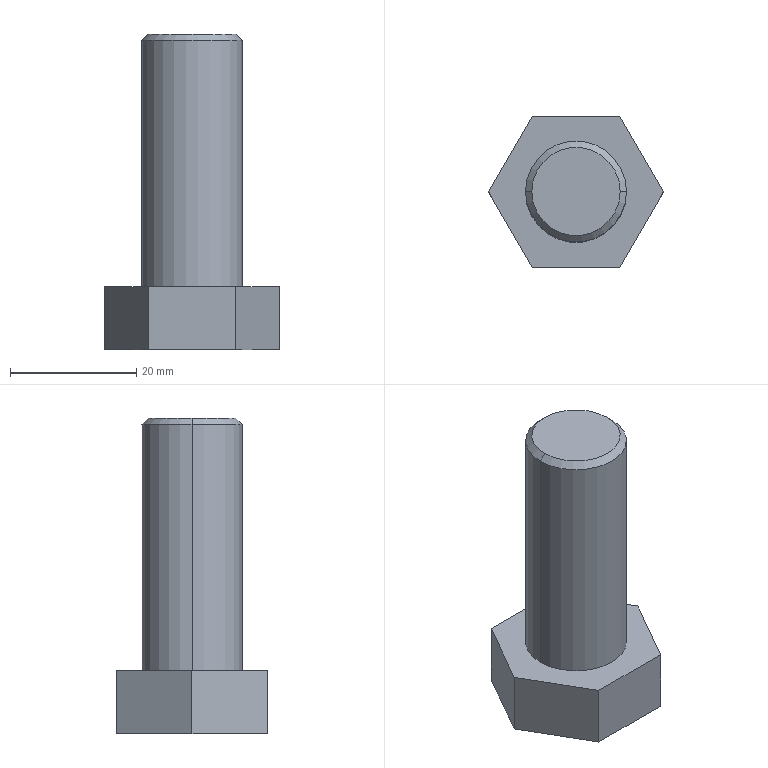Part | STEP file | Bulong M16_4F | 1 solid | 13 faces | box 27.713 x 24 x 50 mm | volume 13007 mm3 | plane 9 | cone 2 | cylinder 2 | commonest cylinder face diameters 16 x2
STEP:
#1=CARTESIAN_POINT('',(0.,0.,0.));
#2=DIRECTION('',(0.,0.,1.));
#3=DIRECTION('',(1.,0.,0.));
#4=AXIS2_PLACEMENT_3D('',#1,#2,#3);
#5=CARTESIAN_POINT('',(7.,0.,40.));
#6=VERTEX_POINT('',#5);
#7=CARTESIAN_POINT('',(-7.,0.,40.));
#8=VERTEX_POINT('',#7);
#9=CARTESIAN_POINT('',(0.,0.,40.));
#10=DIRECTION('',(0.,0.,1.));
#11=DIRECTION('',(1.,0.,0.));
#12=AXIS2_PLACEMENT_3D('',#9,#10,#11);
#13=CIRCLE('',#12,7.);
#14=CARTESIAN_POINT('',(0.,0.,40.));
#15=DIRECTION('',(0.,0.,-1.));
#16=DIRECTION('',(-1.,0.,0.));
#17=AXIS2_PLACEMENT_3D('',#14,#15,#16);
#18=CONICAL_SURFACE('',#17,7.,0.7854);
#19=CARTESIAN_POINT('',(3.142,0.));
#20=DIRECTION('',(-1.,0.));
#21=VECTOR('',#20,1.);
#22=LINE('',#19,#21);
#23=(GEOMETRIC_REPRESENTATION_CONTEXT(2)PARAMETRIC_REPRESENTATION_CONTEXT()REPRESENTATION_CONTEXT('',''));
#24=DEFINITIONAL_REPRESENTATION('',(#22),#23);
#25=PCURVE('',#18,#24);
#26=CARTESIAN_POINT('',(0.,0.,40.));
#27=DIRECTION('',(0.,0.,1.));
#28=DIRECTION('',(1.,0.,0.));
#29=AXIS2_PLACEMENT_3D('',#26,#27,#28);
#30=PLANE('',#29);
#31=CARTESIAN_POINT('',(0.,0.));
#32=DIRECTION('',(1.,0.));
#33=AXIS2_PLACEMENT_2D('',#31,#32);
#34=CIRCLE('',#33,7.);
#35=(GEOMETRIC_REPRESENTATION_CONTEXT(2)PARAMETRIC_REPRESENTATION_CONTEXT()REPRESENTATION_CONTEXT('',''));
#36=DEFINITIONAL_REPRESENTATION('',(#34),#35);
#37=PCURVE('',#30,#36);
#38=SURFACE_CURVE('',#13,(#25,#37),.PCURVE_S1.);
#39=EDGE_CURVE('',#6,#8,#38,.T.);
#40=ORIENTED_EDGE('',*,*,#39,.F.);
#41=CARTESIAN_POINT('',(8.,0.,39.));
#42=VERTEX_POINT('',#41);
#43=CARTESIAN_POINT('',(7.,0.,40.));
#44=DIRECTION('',(0.7071,0.,-0.7071));
#45=VECTOR('',#44,1.);
#46=LINE('',#43,#45);
#47=CARTESIAN_POINT('',(3.142,0.));
#48=DIRECTION('',(0.,1.));
#49=VECTOR('',#48,1.);
#50=LINE('',#47,#49);
#51=(GEOMETRIC_REPRESENTATION_CONTEXT(2)PARAMETRIC_REPRESENTATION_CONTEXT()REPRESENTATION_CONTEXT('',''));
#52=DEFINITIONAL_REPRESENTATION('',(#50),#51);
#53=PCURVE('',#18,#52);
#54=CARTESIAN_POINT('',(0.,0.,40.));
#55=DIRECTION('',(0.,0.,-1.));
#56=DIRECTION('',(-1.,0.,0.));
#57=AXIS2_PLACEMENT_3D('',#54,#55,#56);
#58=CONICAL_SURFACE('',#57,7.,0.7854);
#59=CARTESIAN_POINT('',(3.142,0.));
#60=DIRECTION('',(0.,1.));
#61=VECTOR('',#60,1.);
#62=LINE('',#59,#61);
#63=(GEOMETRIC_REPRESENTATION_CONTEXT(2)PARAMETRIC_REPRESENTATION_CONTEXT()REPRESENTATION_CONTEXT('',''));
#64=DEFINITIONAL_REPRESENTATION('',(#62),#63);
#65=PCURVE('',#58,#64);
#66=SURFACE_CURVE('',#46,(#53,#65),.PCURVE_S1.);
#67=EDGE_CURVE('',#6,#42,#66,.T.);
#68=ORIENTED_EDGE('',*,*,#67,.T.);
#69=CARTESIAN_POINT('',(-8.,0.,39.));
#70=VERTEX_POINT('',#69);
#71=CARTESIAN_POINT('',(0.,0.,39.));
#72=DIRECTION('',(0.,0.,-1.));
#73=DIRECTION('',(1.,0.,0.));
#74=AXIS2_PLACEMENT_3D('',#71,#72,#73);
#75=CIRCLE('',#74,8.);
#76=CARTESIAN_POINT('',(-3.142,1.));
#77=DIRECTION('',(1.,0.));
#78=VECTOR('',#77,1.);
#79=LINE('',#76,#78);
#80=(GEOMETRIC_REPRESENTATION_CONTEXT(2)PARAMETRIC_REPRESENTATION_CONTEXT()REPRESENTATION_CONTEXT('',''));
#81=DEFINITIONAL_REPRESENTATION('',(#79),#80);
#82=PCURVE('',#18,#81);
#83=CARTESIAN_POINT('',(0.,0.,40.));
#84=DIRECTION('',(0.,0.,-1.));
#85=DIRECTION('',(-1.,0.,0.));
#86=AXIS2_PLACEMENT_3D('',#83,#84,#85);
#87=CYLINDRICAL_SURFACE('',#86,8.);
#88=CARTESIAN_POINT('',(-3.142,1.));
#89=DIRECTION('',(1.,0.));
#90=VECTOR('',#89,1.);
#91=LINE('',#88,#90);
#92=(GEOMETRIC_REPRESENTATION_CONTEXT(2)PARAMETRIC_REPRESENTATION_CONTEXT()REPRESENTATION_CONTEXT('',''));
#93=DEFINITIONAL_REPRESENTATION('',(#91),#92);
#94=PCURVE('',#87,#93);
#95=SURFACE_CURVE('',#75,(#82,#94),.PCURVE_S1.);
#96=EDGE_CURVE('',#70,#42,#95,.T.);
#97=ORIENTED_EDGE('',*,*,#96,.F.);
#98=CARTESIAN_POINT('',(-7.,0.,40.));
#99=DIRECTION('',(-0.7071,0.,-0.7071));
#100=VECTOR('',#99,1.);
#101=LINE('',#98,#100);
#102=CARTESIAN_POINT('',(0.,0.));
#103=DIRECTION('',(0.,1.));
#104=VECTOR('',#103,1.);
#105=LINE('',#102,#104);
#106=(GEOMETRIC_REPRESENTATION_CONTEXT(2)PARAMETRIC_REPRESENTATION_CONTEXT()REPRESENTATION_CONTEXT('',''));
#107=DEFINITIONAL_REPRESENTATION('',(#105),#106);
#108=PCURVE('',#18,#107);
#109=CARTESIAN_POINT('',(6.283,0.));
#110=DIRECTION('',(0.,1.));
#111=VECTOR('',#110,1.);
#112=LINE('',#109,#111);
#113=(GEOMETRIC_REPRESENTATION_CONTEXT(2)PARAMETRIC_REPRESENTATION_CONTEXT()REPRESENTATION_CONTEXT('',''));
#114=DEFINITIONAL_REPRESENTATION('',(#112),#113);
#115=PCURVE('',#58,#114);
#116=SURFACE_CURVE('',#101,(#108,#115),.PCURVE_S1.);
#117=EDGE_CURVE('',#8,#70,#116,.T.);
#118=ORIENTED_EDGE('',*,*,#117,.F.);
#119=EDGE_LOOP('',(#40,#68,#97,#118));
#120=FACE_BOUND('',#119,.T.);
#121=ADVANCED_FACE('',(#120),#18,.T.);
#122=ORIENTED_EDGE('',*,*,#96,.T.);
#123=CARTESIAN_POINT('',(8.,0.,0.));
#124=VERTEX_POINT('',#123);
#125=CARTESIAN_POINT('',(8.,0.,40.));
#126=DIRECTION('',(0.,0.,-1.));
#127=VECTOR('',#126,1.);
#128=LINE('',#125,#127);
#129=CARTESIAN_POINT('',(3.142,0.));
#130=DIRECTION('',(0.,1.));
#131=VECTOR('',#130,1.);
#132=LINE('',#129,#131);
#133=(GEOMETRIC_REPRESENTATION_CONTEXT(2)PARAMETRIC_REPRESENTATION_CONTEXT()REPRESENTATION_CONTEXT('',''));
#134=DEFINITIONAL_REPRESENTATION('',(#132),#133);
#135=PCURVE('',#87,#134);
#136=CARTESIAN_POINT('',(0.,0.,40.));
#137=DIRECTION('',(0.,0.,-1.));
#138=DIRECTION('',(-1.,0.,0.));
#139=AXIS2_PLACEMENT_3D('',#136,#137,#138);
#140=CYLINDRICAL_SURFACE('',#139,8.);
#141=CARTESIAN_POINT('',(3.142,0.));
#142=DIRECTION('',(0.,1.));
#143=VECTOR('',#142,1.);
#144=LINE('',#141,#143);
#145=(GEOMETRIC_REPRESENTATION_CONTEXT(2)PARAMETRIC_REPRESENTATION_CONTEXT()REPRESENTATION_CONTEXT('',''));
#146=DEFINITIONAL_REPRESENTATION('',(#144),#145);
#147=PCURVE('',#140,#146);
#148=SURFACE_CURVE('',#128,(#135,#147),.PCURVE_S1.);
#149=EDGE_CURVE('',#42,#124,#148,.T.);
#150=ORIENTED_EDGE('',*,*,#149,.T.);
#151=CARTESIAN_POINT('',(-8.,0.,0.));
#152=VERTEX_POINT('',#151);
#153=CARTESIAN_POINT('',(0.,0.,0.));
#154=DIRECTION('',(0.,0.,1.));
#155=DIRECTION('',(1.,0.,0.));
#156=AXIS2_PLACEMENT_3D('',#153,#154,#155);
#157=CIRCLE('',#156,8.);
#158=CARTESIAN_POINT('',(3.142,40.));
#159=DIRECTION('',(-1.,0.));
#160=VECTOR('',#159,1.);
#161=LINE('',#158,#160);
#162=(GEOMETRIC_REPRESENTATION_CONTEXT(2)PARAMETRIC_REPRESENTATION_CONTEXT()REPRESENTATION_CONTEXT('',''));
#163=DEFINITIONAL_REPRESENTATION('',(#161),#162);
#164=PCURVE('',#87,#163);
#165=CARTESIAN_POINT('',(0.,0.,0.));
#166=DIRECTION('',(0.,0.,1.));
#167=DIRECTION('',(1.,0.,0.));
#168=AXIS2_PLACEMENT_3D('',#165,#166,#167);
#169=PLANE('',#168);
#170=CARTESIAN_POINT('',(0.,0.));
#171=DIRECTION('',(1.,0.));
#172=AXIS2_PLACEMENT_2D('',#170,#171);
#173=CIRCLE('',#172,8.);
#174=(GEOMETRIC_REPRESENTATION_CONTEXT(2)PARAMETRIC_REPRESENTATION_CONTEXT()REPRESENTATION_CONTEXT('',''));
#175=DEFINITIONAL_REPRESENTATION('',(#173),#174);
#176=PCURVE('',#169,#175);
#177=SURFACE_CURVE('',#157,(#164,#176),.PCURVE_S1.);
#178=EDGE_CURVE('',#124,#152,#177,.T.);
#179=ORIENTED_EDGE('',*,*,#178,.T.);
#180=CARTESIAN_POINT('',(-8.,0.,40.));
#181=DIRECTION('',(0.,0.,-1.));
#182=VECTOR('',#181,1.);
#183=LINE('',#180,#182);
#184=CARTESIAN_POINT('',(0.,0.));
#185=DIRECTION('',(0.,1.));
#186=VECTOR('',#185,1.);
#187=LINE('',#184,#186);
#188=(GEOMETRIC_REPRESENTATION_CONTEXT(2)PARAMETRIC_REPRESENTATION_CONTEXT()REPRESENTATION_CONTEXT('',''));
#189=DEFINITIONAL_REPRESENTATION('',(#187),#188);
#190=PCURVE('',#87,#189);
#191=CARTESIAN_POINT('',(6.283,0.));
#192=DIRECTION('',(0.,1.));
#193=VECTOR('',#192,1.);
#194=LINE('',#191,#193);
#195=(GEOMETRIC_REPRESENTATION_CONTEXT(2)PARAMETRIC_REPRESENTATION_CONTEXT()REPRESENTATION_CONTEXT('',''));
#196=DEFINITIONAL_REPRESENTATION('',(#194),#195);
#197=PCURVE('',#140,#196);
#198=SURFACE_CURVE('',#183,(#190,#197),.PCURVE_S1.);
#199=EDGE_CURVE('',#70,#152,#198,.T.);
#200=ORIENTED_EDGE('',*,*,#199,.F.);
#201=EDGE_LOOP('',(#122,#150,#179,#200));
#202=FACE_BOUND('',#201,.T.);
#203=ADVANCED_FACE('',(#202),#87,.T.);
#204=CARTESIAN_POINT('',(6.928,-12.,0.));
#205=VERTEX_POINT('',#204);
#206=CARTESIAN_POINT('',(13.856,0.,0.));
#207=VERTEX_POINT('',#206);
#208=CARTESIAN_POINT('',(6.928,-12.,0.));
#209=DIRECTION('',(0.5,0.866,0.));
#210=VECTOR('',#209,1.);
#211=LINE('',#208,#210);
#212=CARTESIAN_POINT('',(6.928,-12.));
#213=DIRECTION('',(0.5,0.866));
#214=VECTOR('',#213,1.);
#215=LINE('',#212,#214);
#216=(GEOMETRIC_REPRESENTATION_CONTEXT(2)PARAMETRIC_REPRESENTATION_CONTEXT()REPRESENTATION_CONTEXT('',''));
#217=DEFINITIONAL_REPRESENTATION('',(#215),#216);
#218=PCURVE('',#169,#217);
#219=CARTESIAN_POINT('',(6.928,-12.,-10.));
#220=DIRECTION('',(0.866,-0.5,0.));
#221=DIRECTION('',(0.5,0.866,0.));
#222=AXIS2_PLACEMENT_3D('',#219,#220,#221);
#223=PLANE('',#222);
#224=CARTESIAN_POINT('',(0.,10.));
#225=DIRECTION('',(1.,0.));
#226=VECTOR('',#225,1.);
#227=LINE('',#224,#226);
#228=(GEOMETRIC_REPRESENTATION_CONTEXT(2)PARAMETRIC_REPRESENTATION_CONTEXT()REPRESENTATION_CONTEXT('',''));
#229=DEFINITIONAL_REPRESENTATION('',(#227),#228);
#230=PCURVE('',#223,#229);
#231=SURFACE_CURVE('',#211,(#218,#230),.PCURVE_S1.);
#232=EDGE_CURVE('',#205,#207,#231,.T.);
#233=ORIENTED_EDGE('',*,*,#232,.T.);
#234=CARTESIAN_POINT('',(6.928,12.,0.));
#235=VERTEX_POINT('',#234);
#236=CARTESIAN_POINT('',(13.856,0.,0.));
#237=DIRECTION('',(-0.5,0.866,0.));
#238=VECTOR('',#237,1.);
#239=LINE('',#236,#238);
#240=CARTESIAN_POINT('',(13.856,0.));
#241=DIRECTION('',(-0.5,0.866));
#242=VECTOR('',#241,1.);
#243=LINE('',#240,#242);
#244=(GEOMETRIC_REPRESENTATION_CONTEXT(2)PARAMETRIC_REPRESENTATION_CONTEXT()REPRESENTATION_CONTEXT('',''));
#245=DEFINITIONAL_REPRESENTATION('',(#243),#244);
#246=PCURVE('',#169,#245);
#247=CARTESIAN_POINT('',(13.856,0.,-10.));
#248=DIRECTION('',(0.866,0.5,0.));
#249=DIRECTION('',(-0.5,0.866,0.));
#250=AXIS2_PLACEMENT_3D('',#247,#248,#249);
#251=PLANE('',#250);
#252=CARTESIAN_POINT('',(0.,10.));
#253=DIRECTION('',(1.,0.));
#254=VECTOR('',#253,1.);
#255=LINE('',#252,#254);
#256=(GEOMETRIC_REPRESENTATION_CONTEXT(2)PARAMETRIC_REPRESENTATION_CONTEXT()REPRESENTATION_CONTEXT('',''));
#257=DEFINITIONAL_REPRESENTATION('',(#255),#256);
#258=PCURVE('',#251,#257);
#259=SURFACE_CURVE('',#239,(#246,#258),.PCURVE_S1.);
#260=EDGE_CURVE('',#207,#235,#259,.T.);
#261=ORIENTED_EDGE('',*,*,#260,.T.);
#262=CARTESIAN_POINT('',(-6.928,12.,0.));
#263=VERTEX_POINT('',#262);
#264=CARTESIAN_POINT('',(6.928,12.,0.));
#265=DIRECTION('',(-1.,0.,0.));
#266=VECTOR('',#265,1.);
#267=LINE('',#264,#266);
#268=CARTESIAN_POINT('',(6.928,12.));
#269=DIRECTION('',(-1.,0.));
#270=VECTOR('',#269,1.);
#271=LINE('',#268,#270);
#272=(GEOMETRIC_REPRESENTATION_CONTEXT(2)PARAMETRIC_REPRESENTATION_CONTEXT()REPRESENTATION_CONTEXT('',''));
#273=DEFINITIONAL_REPRESENTATION('',(#271),#272);
#274=PCURVE('',#169,#273);
#275=CARTESIAN_POINT('',(6.928,12.,-10.));
#276=DIRECTION('',(0.,1.,0.));
#277=DIRECTION('',(-1.,0.,0.));
#278=AXIS2_PLACEMENT_3D('',#275,#276,#277);
#279=PLANE('',#278);
#280=CARTESIAN_POINT('',(0.,10.));
#281=DIRECTION('',(1.,0.));
#282=VECTOR('',#281,1.);
#283=LINE('',#280,#282);
#284=(GEOMETRIC_REPRESENTATION_CONTEXT(2)PARAMETRIC_REPRESENTATION_CONTEXT()REPRESENTATION_CONTEXT('',''));
#285=DEFINITIONAL_REPRESENTATION('',(#283),#284);
#286=PCURVE('',#279,#285);
#287=SURFACE_CURVE('',#267,(#274,#286),.PCURVE_S1.);
#288=EDGE_CURVE('',#235,#263,#287,.T.);
#289=ORIENTED_EDGE('',*,*,#288,.T.);
#290=CARTESIAN_POINT('',(-13.856,0.,0.));
#291=VERTEX_POINT('',#290);
#292=CARTESIAN_POINT('',(-6.928,12.,0.));
#293=DIRECTION('',(-0.5,-0.866,0.));
#294=VECTOR('',#293,1.);
#295=LINE('',#292,#294);
#296=CARTESIAN_POINT('',(-6.928,12.));
#297=DIRECTION('',(-0.5,-0.866));
#298=VECTOR('',#297,1.);
#299=LINE('',#296,#298);
#300=(GEOMETRIC_REPRESENTATION_CONTEXT(2)PARAMETRIC_REPRESENTATION_CONTEXT()REPRESENTATION_CONTEXT('',''));
#301=DEFINITIONAL_REPRESENTATION('',(#299),#300);
#302=PCURVE('',#169,#301);
#303=CARTESIAN_POINT('',(-6.928,12.,-10.));
#304=DIRECTION('',(-0.866,0.5,0.));
#305=DIRECTION('',(-0.5,-0.866,0.));
#306=AXIS2_PLACEMENT_3D('',#303,#304,#305);
#307=PLANE('',#306);
#308=CARTESIAN_POINT('',(0.,10.));
#309=DIRECTION('',(1.,0.));
#310=VECTOR('',#309,1.);
#311=LINE('',#308,#310);
#312=(GEOMETRIC_REPRESENTATION_CONTEXT(2)PARAMETRIC_REPRESENTATION_CONTEXT()REPRESENTATION_CONTEXT('',''));
#313=DEFINITIONAL_REPRESENTATION('',(#311),#312);
#314=PCURVE('',#307,#313);
#315=SURFACE_CURVE('',#295,(#302,#314),.PCURVE_S1.);
#316=EDGE_CURVE('',#263,#291,#315,.T.);
#317=ORIENTED_EDGE('',*,*,#316,.T.);
#318=CARTESIAN_POINT('',(-6.928,-12.,0.));
#319=VERTEX_POINT('',#318);
#320=CARTESIAN_POINT('',(-13.856,0.,0.));
#321=DIRECTION('',(0.5,-0.866,0.));
#322=VECTOR('',#321,1.);
#323=LINE('',#320,#322);
#324=CARTESIAN_POINT('',(-13.856,0.));
#325=DIRECTION('',(0.5,-0.866));
#326=VECTOR('',#325,1.);
#327=LINE('',#324,#326);
#328=(GEOMETRIC_REPRESENTATION_CONTEXT(2)PARAMETRIC_REPRESENTATION_CONTEXT()REPRESENTATION_CONTEXT('',''));
#329=DEFINITIONAL_REPRESENTATION('',(#327),#328);
#330=PCURVE('',#169,#329);
#331=CARTESIAN_POINT('',(-13.856,0.,-10.));
#332=DIRECTION('',(-0.866,-0.5,0.));
#333=DIRECTION('',(0.5,-0.866,0.));
#334=AXIS2_PLACEMENT_3D('',#331,#332,#333);
#335=PLANE('',#334);
#336=CARTESIAN_POINT('',(0.,10.));
#337=DIRECTION('',(1.,0.));
#338=VECTOR('',#337,1.);
#339=LINE('',#336,#338);
#340=(GEOMETRIC_REPRESENTATION_CONTEXT(2)PARAMETRIC_REPRESENTATION_CONTEXT()REPRESENTATION_CONTEXT('',''));
#341=DEFINITIONAL_REPRESENTATION('',(#339),#340);
#342=PCURVE('',#335,#341);
#343=SURFACE_CURVE('',#323,(#330,#342),.PCURVE_S1.);
#344=EDGE_CURVE('',#291,#319,#343,.T.);
#345=ORIENTED_EDGE('',*,*,#344,.T.);
#346=CARTESIAN_POINT('',(-6.928,-12.,0.));
#347=DIRECTION('',(1.,0.,0.));
#348=VECTOR('',#347,1.);
#349=LINE('',#346,#348);
#350=CARTESIAN_POINT('',(-6.928,-12.));
#351=DIRECTION('',(1.,0.));
#352=VECTOR('',#351,1.);
#353=LINE('',#350,#352);
#354=(GEOMETRIC_REPRESENTATION_CONTEXT(2)PARAMETRIC_REPRESENTATION_CONTEXT()REPRESENTATION_CONTEXT('',''));
#355=DEFINITIONAL_REPRESENTATION('',(#353),#354);
#356=PCURVE('',#169,#355);
#357=CARTESIAN_POINT('',(-6.928,-12.,-10.));
#358=DIRECTION('',(0.,-1.,0.));
#359=DIRECTION('',(0.,0.,-1.));
#360=AXIS2_PLACEMENT_3D('',#357,#358,#359);
#361=PLANE('',#360);
#362=CARTESIAN_POINT('',(-10.,0.));
#363=DIRECTION('',(0.,1.));
#364=VECTOR('',#363,1.);
#365=LINE('',#362,#364);
#366=(GEOMETRIC_REPRESENTATION_CONTEXT(2)PARAMETRIC_REPRESENTATION_CONTEXT()REPRESENTATION_CONTEXT('',''));
#367=DEFINITIONAL_REPRESENTATION('',(#365),#366);
#368=PCURVE('',#361,#367);
#369=SURFACE_CURVE('',#349,(#356,#368),.PCURVE_S1.);
#370=EDGE_CURVE('',#319,#205,#369,.T.);
#371=ORIENTED_EDGE('',*,*,#370,.T.);
#372=EDGE_LOOP('',(#233,#261,#289,#317,#345,#371));
#373=FACE_BOUND('',#372,.T.);
#374=CARTESIAN_POINT('',(0.,0.,0.));
#375=DIRECTION('',(0.,0.,1.));
#376=DIRECTION('',(1.,0.,0.));
#377=AXIS2_PLACEMENT_3D('',#374,#375,#376);
#378=CIRCLE('',#377,8.);
#379=CARTESIAN_POINT('',(0.,0.));
#380=DIRECTION('',(1.,0.));
#381=AXIS2_PLACEMENT_2D('',#379,#380);
#382=CIRCLE('',#381,8.);
#383=(GEOMETRIC_REPRESENTATION_CONTEXT(2)PARAMETRIC_REPRESENTATION_CONTEXT()REPRESENTATION_CONTEXT('',''));
#384=DEFINITIONAL_REPRESENTATION('',(#382),#383);
#385=PCURVE('',#169,#384);
#386=CARTESIAN_POINT('',(9.425,40.));
#387=DIRECTION('',(-1.,0.));
#388=VECTOR('',#387,1.);
#389=LINE('',#386,#388);
#390=(GEOMETRIC_REPRESENTATION_CONTEXT(2)PARAMETRIC_REPRESENTATION_CONTEXT()REPRESENTATION_CONTEXT('',''));
#391=DEFINITIONAL_REPRESENTATION('',(#389),#390);
#392=PCURVE('',#140,#391);
#393=SURFACE_CURVE('',#378,(#385,#392),.PCURVE_S1.);
#394=EDGE_CURVE('',#152,#124,#393,.T.);
#395=ORIENTED_EDGE('',*,*,#394,.F.);
#396=ORIENTED_EDGE('',*,*,#178,.F.);
#397=EDGE_LOOP('',(#395,#396));
#398=FACE_BOUND('',#397,.T.);
#399=ADVANCED_FACE('',(#373,#398),#169,.T.);
#400=ORIENTED_EDGE('',*,*,#232,.F.);
#401=CARTESIAN_POINT('',(6.928,-12.,-10.));
#402=VERTEX_POINT('',#401);
#403=CARTESIAN_POINT('',(6.928,-12.,-10.));
#404=DIRECTION('',(0.,0.,1.));
#405=VECTOR('',#404,1.);
#406=LINE('',#403,#405);
#407=CARTESIAN_POINT('',(0.,0.));
#408=DIRECTION('',(0.,1.));
#409=VECTOR('',#408,1.);
#410=LINE('',#407,#409);
#411=(GEOMETRIC_REPRESENTATION_CONTEXT(2)PARAMETRIC_REPRESENTATION_CONTEXT()REPRESENTATION_CONTEXT('',''));
#412=DEFINITIONAL_REPRESENTATION('',(#410),#411);
#413=PCURVE('',#223,#412);
#414=CARTESIAN_POINT('',(0.,13.856));
#415=DIRECTION('',(-1.,0.));
#416=VECTOR('',#415,1.);
#417=LINE('',#414,#416);
#418=(GEOMETRIC_REPRESENTATION_CONTEXT(2)PARAMETRIC_REPRESENTATION_CONTEXT()REPRESENTATION_CONTEXT('',''));
#419=DEFINITIONAL_REPRESENTATION('',(#417),#418);
#420=PCURVE('',#361,#419);
#421=SURFACE_CURVE('',#406,(#413,#420),.PCURVE_S1.);
#422=EDGE_CURVE('',#402,#205,#421,.T.);
#423=ORIENTED_EDGE('',*,*,#422,.F.);
#424=CARTESIAN_POINT('',(13.856,0.,-10.));
#425=VERTEX_POINT('',#424);
#426=CARTESIAN_POINT('',(6.928,-12.,-10.));
#427=DIRECTION('',(0.5,0.866,0.));
#428=VECTOR('',#427,1.);
#429=LINE('',#426,#428);
#430=CARTESIAN_POINT('',(0.,0.));
#431=DIRECTION('',(1.,0.));
#432=VECTOR('',#431,1.);
#433=LINE('',#430,#432);
#434=(GEOMETRIC_REPRESENTATION_CONTEXT(2)PARAMETRIC_REPRESENTATION_CONTEXT()REPRESENTATION_CONTEXT('',''));
#435=DEFINITIONAL_REPRESENTATION('',(#433),#434);
#436=PCURVE('',#223,#435);
#437=CARTESIAN_POINT('',(0.,0.,-10.));
#438=DIRECTION('',(0.,0.,1.));
#439=DIRECTION('',(1.,0.,0.));
#440=AXIS2_PLACEMENT_3D('',#437,#438,#439);
#441=PLANE('',#440);
#442=CARTESIAN_POINT('',(6.928,-12.));
#443=DIRECTION('',(0.5,0.866));
#444=VECTOR('',#443,1.);
#445=LINE('',#442,#444);
#446=(GEOMETRIC_REPRESENTATION_CONTEXT(2)PARAMETRIC_REPRESENTATION_CONTEXT()REPRESENTATION_CONTEXT('',''));
#447=DEFINITIONAL_REPRESENTATION('',(#445),#446);
#448=PCURVE('',#441,#447);
#449=SURFACE_CURVE('',#429,(#436,#448),.PCURVE_S1.);
#450=EDGE_CURVE('',#402,#425,#449,.T.);
#451=ORIENTED_EDGE('',*,*,#450,.T.);
#452=CARTESIAN_POINT('',(13.856,0.,-10.));
#453=DIRECTION('',(0.,0.,1.));
#454=VECTOR('',#453,1.);
#455=LINE('',#452,#454);
#456=CARTESIAN_POINT('',(13.856,0.));
#457=DIRECTION('',(0.,1.));
#458=VECTOR('',#457,1.);
#459=LINE('',#456,#458);
#460=(GEOMETRIC_REPRESENTATION_CONTEXT(2)PARAMETRIC_REPRESENTATION_CONTEXT()REPRESENTATION_CONTEXT('',''));
#461=DEFINITIONAL_REPRESENTATION('',(#459),#460);
#462=PCURVE('',#223,#461);
#463=CARTESIAN_POINT('',(0.,0.));
#464=DIRECTION('',(0.,1.));
#465=VECTOR('',#464,1.);
#466=LINE('',#463,#465);
#467=(GEOMETRIC_REPRESENTATION_CONTEXT(2)PARAMETRIC_REPRESENTATION_CONTEXT()REPRESENTATION_CONTEXT('',''));
#468=DEFINITIONAL_REPRESENTATION('',(#466),#467);
#469=PCURVE('',#251,#468);
#470=SURFACE_CURVE('',#455,(#462,#469),.PCURVE_S1.);
#471=EDGE_CURVE('',#425,#207,#470,.T.);
#472=ORIENTED_EDGE('',*,*,#471,.T.);
#473=EDGE_LOOP('',(#400,#423,#451,#472));
#474=FACE_BOUND('',#473,.T.);
#475=ADVANCED_FACE('',(#474),#223,.T.);
#476=ORIENTED_EDGE('',*,*,#370,.F.);
#477=CARTESIAN_POINT('',(-6.928,-12.,-10.));
#478=VERTEX_POINT('',#477);
#479=CARTESIAN_POINT('',(-6.928,-12.,-10.));
#480=DIRECTION('',(0.,0.,1.));
#481=VECTOR('',#480,1.);
#482=LINE('',#479,#481);
#483=CARTESIAN_POINT('',(0.,0.));
#484=DIRECTION('',(-1.,0.));
#485=VECTOR('',#484,1.);
#486=LINE('',#483,#485);
#487=(GEOMETRIC_REPRESENTATION_CONTEXT(2)PARAMETRIC_REPRESENTATION_CONTEXT()REPRESENTATION_CONTEXT('',''));
#488=DEFINITIONAL_REPRESENTATION('',(#486),#487);
#489=PCURVE('',#361,#488);
#490=CARTESIAN_POINT('',(13.856,0.));
#491=DIRECTION('',(0.,1.));
#492=VECTOR('',#491,1.);
#493=LINE('',#490,#492);
#494=(GEOMETRIC_REPRESENTATION_CONTEXT(2)PARAMETRIC_REPRESENTATION_CONTEXT()REPRESENTATION_CONTEXT('',''));
#495=DEFINITIONAL_REPRESENTATION('',(#493),#494);
#496=PCURVE('',#335,#495);
#497=SURFACE_CURVE('',#482,(#489,#496),.PCURVE_S1.);
#498=EDGE_CURVE('',#478,#319,#497,.T.);
#499=ORIENTED_EDGE('',*,*,#498,.F.);
#500=CARTESIAN_POINT('',(-6.928,-12.,-10.));
#501=DIRECTION('',(1.,0.,0.));
#502=VECTOR('',#501,1.);
#503=LINE('',#500,#502);
#504=CARTESIAN_POINT('',(0.,0.));
#505=DIRECTION('',(0.,1.));
#506=VECTOR('',#505,1.);
#507=LINE('',#504,#506);
#508=(GEOMETRIC_REPRESENTATION_CONTEXT(2)PARAMETRIC_REPRESENTATION_CONTEXT()REPRESENTATION_CONTEXT('',''));
#509=DEFINITIONAL_REPRESENTATION('',(#507),#508);
#510=PCURVE('',#361,#509);
#511=CARTESIAN_POINT('',(-6.928,-12.));
#512=DIRECTION('',(1.,0.));
#513=VECTOR('',#512,1.);
#514=LINE('',#511,#513);
#515=(GEOMETRIC_REPRESENTATION_CONTEXT(2)PARAMETRIC_REPRESENTATION_CONTEXT()REPRESENTATION_CONTEXT('',''));
#516=DEFINITIONAL_REPRESENTATION('',(#514),#515);
#517=PCURVE('',#441,#516);
#518=SURFACE_CURVE('',#503,(#510,#517),.PCURVE_S1.);
#519=EDGE_CURVE('',#478,#402,#518,.T.);
#520=ORIENTED_EDGE('',*,*,#519,.T.);
#521=ORIENTED_EDGE('',*,*,#422,.T.);
#522=EDGE_LOOP('',(#476,#499,#520,#521));
#523=FACE_BOUND('',#522,.T.);
#524=ADVANCED_FACE('',(#523),#361,.T.);
#525=ORIENTED_EDGE('',*,*,#344,.F.);
#526=CARTESIAN_POINT('',(-13.856,0.,-10.));
#527=VERTEX_POINT('',#526);
#528=CARTESIAN_POINT('',(-13.856,0.,-10.));
#529=DIRECTION('',(0.,0.,1.));
#530=VECTOR('',#529,1.);
#531=LINE('',#528,#530);
#532=CARTESIAN_POINT('',(0.,0.));
#533=DIRECTION('',(0.,1.));
#534=VECTOR('',#533,1.);
#535=LINE('',#532,#534);
#536=(GEOMETRIC_REPRESENTATION_CONTEXT(2)PARAMETRIC_REPRESENTATION_CONTEXT()REPRESENTATION_CONTEXT('',''));
#537=DEFINITIONAL_REPRESENTATION('',(#535),#536);
#538=PCURVE('',#335,#537);
#539=CARTESIAN_POINT('',(13.856,0.));
#540=DIRECTION('',(0.,1.));
#541=VECTOR('',#540,1.);
#542=LINE('',#539,#541);
#543=(GEOMETRIC_REPRESENTATION_CONTEXT(2)PARAMETRIC_REPRESENTATION_CONTEXT()REPRESENTATION_CONTEXT('',''));
#544=DEFINITIONAL_REPRESENTATION('',(#542),#543);
#545=PCURVE('',#307,#544);
#546=SURFACE_CURVE('',#531,(#538,#545),.PCURVE_S1.);
#547=EDGE_CURVE('',#527,#291,#546,.T.);
#548=ORIENTED_EDGE('',*,*,#547,.F.);
#549=CARTESIAN_POINT('',(-13.856,0.,-10.));
#550=DIRECTION('',(0.5,-0.866,0.));
#551=VECTOR('',#550,1.);
#552=LINE('',#549,#551);
#553=CARTESIAN_POINT('',(0.,0.));
#554=DIRECTION('',(1.,0.));
#555=VECTOR('',#554,1.);
#556=LINE('',#553,#555);
#557=(GEOMETRIC_REPRESENTATION_CONTEXT(2)PARAMETRIC_REPRESENTATION_CONTEXT()REPRESENTATION_CONTEXT('',''));
#558=DEFINITIONAL_REPRESENTATION('',(#556),#557);
#559=PCURVE('',#335,#558);
#560=CARTESIAN_POINT('',(-13.856,0.));
#561=DIRECTION('',(0.5,-0.866));
#562=VECTOR('',#561,1.);
#563=LINE('',#560,#562);
#564=(GEOMETRIC_REPRESENTATION_CONTEXT(2)PARAMETRIC_REPRESENTATION_CONTEXT()REPRESENTATION_CONTEXT('',''));
#565=DEFINITIONAL_REPRESENTATION('',(#563),#564);
#566=PCURVE('',#441,#565);
#567=SURFACE_CURVE('',#552,(#559,#566),.PCURVE_S1.);
#568=EDGE_CURVE('',#527,#478,#567,.T.);
#569=ORIENTED_EDGE('',*,*,#568,.T.);
#570=ORIENTED_EDGE('',*,*,#498,.T.);
#571=EDGE_LOOP('',(#525,#548,#569,#570));
#572=FACE_BOUND('',#571,.T.);
#573=ADVANCED_FACE('',(#572),#335,.T.);
#574=ORIENTED_EDGE('',*,*,#316,.F.);
#575=CARTESIAN_POINT('',(-6.928,12.,-10.));
#576=VERTEX_POINT('',#575);
#577=CARTESIAN_POINT('',(-6.928,12.,-10.));
#578=DIRECTION('',(0.,0.,1.));
#579=VECTOR('',#578,1.);
#580=LINE('',#577,#579);
#581=CARTESIAN_POINT('',(0.,0.));
#582=DIRECTION('',(0.,1.));
#583=VECTOR('',#582,1.);
#584=LINE('',#581,#583);
#585=(GEOMETRIC_REPRESENTATION_CONTEXT(2)PARAMETRIC_REPRESENTATION_CONTEXT()REPRESENTATION_CONTEXT('',''));
#586=DEFINITIONAL_REPRESENTATION('',(#584),#585);
#587=PCURVE('',#307,#586);
#588=CARTESIAN_POINT('',(13.856,0.));
#589=DIRECTION('',(0.,1.));
#590=VECTOR('',#589,1.);
#591=LINE('',#588,#590);
#592=(GEOMETRIC_REPRESENTATION_CONTEXT(2)PARAMETRIC_REPRESENTATION_CONTEXT()REPRESENTATION_CONTEXT('',''));
#593=DEFINITIONAL_REPRESENTATION('',(#591),#592);
#594=PCURVE('',#279,#593);
#595=SURFACE_CURVE('',#580,(#587,#594),.PCURVE_S1.);
#596=EDGE_CURVE('',#576,#263,#595,.T.);
#597=ORIENTED_EDGE('',*,*,#596,.F.);
#598=CARTESIAN_POINT('',(-6.928,12.,-10.));
#599=DIRECTION('',(-0.5,-0.866,0.));
#600=VECTOR('',#599,1.);
#601=LINE('',#598,#600);
#602=CARTESIAN_POINT('',(0.,0.));
#603=DIRECTION('',(1.,0.));
#604=VECTOR('',#603,1.);
#605=LINE('',#602,#604);
#606=(GEOMETRIC_REPRESENTATION_CONTEXT(2)PARAMETRIC_REPRESENTATION_CONTEXT()REPRESENTATION_CONTEXT('',''));
#607=DEFINITIONAL_REPRESENTATION('',(#605),#606);
#608=PCURVE('',#307,#607);
#609=CARTESIAN_POINT('',(-6.928,12.));
#610=DIRECTION('',(-0.5,-0.866));
#611=VECTOR('',#610,1.);
#612=LINE('',#609,#611);
#613=(GEOMETRIC_REPRESENTATION_CONTEXT(2)PARAMETRIC_REPRESENTATION_CONTEXT()REPRESENTATION_CONTEXT('',''));
#614=DEFINITIONAL_REPRESENTATION('',(#612),#613);
#615=PCURVE('',#441,#614);
#616=SURFACE_CURVE('',#601,(#608,#615),.PCURVE_S1.);
#617=EDGE_CURVE('',#576,#527,#616,.T.);
#618=ORIENTED_EDGE('',*,*,#617,.T.);
#619=ORIENTED_EDGE('',*,*,#547,.T.);
#620=EDGE_LOOP('',(#574,#597,#618,#619));
#621=FACE_BOUND('',#620,.T.);
#622=ADVANCED_FACE('',(#621),#307,.T.);
#623=ORIENTED_EDGE('',*,*,#288,.F.);
#624=CARTESIAN_POINT('',(6.928,12.,-10.));
#625=VERTEX_POINT('',#624);
#626=CARTESIAN_POINT('',(6.928,12.,-10.));
#627=DIRECTION('',(0.,0.,1.));
#628=VECTOR('',#627,1.);
#629=LINE('',#626,#628);
#630=CARTESIAN_POINT('',(0.,0.));
#631=DIRECTION('',(0.,1.));
#632=VECTOR('',#631,1.);
#633=LINE('',#630,#632);
#634=(GEOMETRIC_REPRESENTATION_CONTEXT(2)PARAMETRIC_REPRESENTATION_CONTEXT()REPRESENTATION_CONTEXT('',''));
#635=DEFINITIONAL_REPRESENTATION('',(#633),#634);
#636=PCURVE('',#279,#635);
#637=CARTESIAN_POINT('',(13.856,0.));
#638=DIRECTION('',(0.,1.));
#639=VECTOR('',#638,1.);
#640=LINE('',#637,#639);
#641=(GEOMETRIC_REPRESENTATION_CONTEXT(2)PARAMETRIC_REPRESENTATION_CONTEXT()REPRESENTATION_CONTEXT('',''));
#642=DEFINITIONAL_REPRESENTATION('',(#640),#641);
#643=PCURVE('',#251,#642);
#644=SURFACE_CURVE('',#629,(#636,#643),.PCURVE_S1.);
#645=EDGE_CURVE('',#625,#235,#644,.T.);
#646=ORIENTED_EDGE('',*,*,#645,.F.);
#647=CARTESIAN_POINT('',(6.928,12.,-10.));
#648=DIRECTION('',(-1.,0.,0.));
#649=VECTOR('',#648,1.);
#650=LINE('',#647,#649);
#651=CARTESIAN_POINT('',(0.,0.));
#652=DIRECTION('',(1.,0.));
#653=VECTOR('',#652,1.);
#654=LINE('',#651,#653);
#655=(GEOMETRIC_REPRESENTATION_CONTEXT(2)PARAMETRIC_REPRESENTATION_CONTEXT()REPRESENTATION_CONTEXT('',''));
#656=DEFINITIONAL_REPRESENTATION('',(#654),#655);
#657=PCURVE('',#279,#656);
#658=CARTESIAN_POINT('',(6.928,12.));
#659=DIRECTION('',(-1.,0.));
#660=VECTOR('',#659,1.);
#661=LINE('',#658,#660);
#662=(GEOMETRIC_REPRESENTATION_CONTEXT(2)PARAMETRIC_REPRESENTATION_CONTEXT()REPRESENTATION_CONTEXT('',''));
#663=DEFINITIONAL_REPRESENTATION('',(#661),#662);
#664=PCURVE('',#441,#663);
#665=SURFACE_CURVE('',#650,(#657,#664),.PCURVE_S1.);
#666=EDGE_CURVE('',#625,#576,#665,.T.);
#667=ORIENTED_EDGE('',*,*,#666,.T.);
#668=ORIENTED_EDGE('',*,*,#596,.T.);
#669=EDGE_LOOP('',(#623,#646,#667,#668));
#670=FACE_BOUND('',#669,.T.);
#671=ADVANCED_FACE('',(#670),#279,.T.);
#672=ORIENTED_EDGE('',*,*,#260,.F.);
#673=ORIENTED_EDGE('',*,*,#471,.F.);
#674=CARTESIAN_POINT('',(13.856,0.,-10.));
#675=DIRECTION('',(-0.5,0.866,0.));
#676=VECTOR('',#675,1.);
#677=LINE('',#674,#676);
#678=CARTESIAN_POINT('',(0.,0.));
#679=DIRECTION('',(1.,0.));
#680=VECTOR('',#679,1.);
#681=LINE('',#678,#680);
#682=(GEOMETRIC_REPRESENTATION_CONTEXT(2)PARAMETRIC_REPRESENTATION_CONTEXT()REPRESENTATION_CONTEXT('',''));
#683=DEFINITIONAL_REPRESENTATION('',(#681),#682);
#684=PCURVE('',#251,#683);
#685=CARTESIAN_POINT('',(13.856,0.));
#686=DIRECTION('',(-0.5,0.866));
#687=VECTOR('',#686,1.);
#688=LINE('',#685,#687);
#689=(GEOMETRIC_REPRESENTATION_CONTEXT(2)PARAMETRIC_REPRESENTATION_CONTEXT()REPRESENTATION_CONTEXT('',''));
#690=DEFINITIONAL_REPRESENTATION('',(#688),#689);
#691=PCURVE('',#441,#690);
#692=SURFACE_CURVE('',#677,(#684,#691),.PCURVE_S1.);
#693=EDGE_CURVE('',#425,#625,#692,.T.);
#694=ORIENTED_EDGE('',*,*,#693,.T.);
#695=ORIENTED_EDGE('',*,*,#645,.T.);
#696=EDGE_LOOP('',(#672,#673,#694,#695));
#697=FACE_BOUND('',#696,.T.);
#698=ADVANCED_FACE('',(#697),#251,.T.);
#699=ORIENTED_EDGE('',*,*,#450,.F.);
#700=ORIENTED_EDGE('',*,*,#519,.F.);
#701=ORIENTED_EDGE('',*,*,#568,.F.);
#702=ORIENTED_EDGE('',*,*,#617,.F.);
#703=ORIENTED_EDGE('',*,*,#666,.F.);
#704=ORIENTED_EDGE('',*,*,#693,.F.);
#705=EDGE_LOOP('',(#699,#700,#701,#702,#703,#704));
#706=FACE_BOUND('',#705,.T.);
#707=ADVANCED_FACE('',(#706),#441,.F.);
#708=ORIENTED_EDGE('',*,*,#149,.F.);
#709=CARTESIAN_POINT('',(0.,0.,39.));
#710=DIRECTION('',(0.,0.,-1.));
#711=DIRECTION('',(1.,0.,0.));
#712=AXIS2_PLACEMENT_3D('',#709,#710,#711);
#713=CIRCLE('',#712,8.);
#714=CARTESIAN_POINT('',(3.142,1.));
#715=DIRECTION('',(1.,0.));
#716=VECTOR('',#715,1.);
#717=LINE('',#714,#716);
#718=(GEOMETRIC_REPRESENTATION_CONTEXT(2)PARAMETRIC_REPRESENTATION_CONTEXT()REPRESENTATION_CONTEXT('',''));
#719=DEFINITIONAL_REPRESENTATION('',(#717),#718);
#720=PCURVE('',#140,#719);
#721=CARTESIAN_POINT('',(3.142,1.));
#722=DIRECTION('',(1.,0.));
#723=VECTOR('',#722,1.);
#724=LINE('',#721,#723);
#725=(GEOMETRIC_REPRESENTATION_CONTEXT(2)PARAMETRIC_REPRESENTATION_CONTEXT()REPRESENTATION_CONTEXT('',''));
#726=DEFINITIONAL_REPRESENTATION('',(#724),#725);
#727=PCURVE('',#58,#726);
#728=SURFACE_CURVE('',#713,(#720,#727),.PCURVE_S1.);
#729=EDGE_CURVE('',#42,#70,#728,.T.);
#730=ORIENTED_EDGE('',*,*,#729,.T.);
#731=ORIENTED_EDGE('',*,*,#199,.T.);
#732=ORIENTED_EDGE('',*,*,#394,.T.);
#733=EDGE_LOOP('',(#708,#730,#731,#732));
#734=FACE_BOUND('',#733,.T.);
#735=ADVANCED_FACE('',(#734),#140,.T.);
#736=CARTESIAN_POINT('',(0.,0.,40.));
#737=DIRECTION('',(0.,0.,1.));
#738=DIRECTION('',(1.,0.,0.));
#739=AXIS2_PLACEMENT_3D('',#736,#737,#738);
#740=CIRCLE('',#739,7.);
#741=CARTESIAN_POINT('',(0.,0.));
#742=DIRECTION('',(1.,0.));
#743=AXIS2_PLACEMENT_2D('',#741,#742);
#744=CIRCLE('',#743,7.);
#745=(GEOMETRIC_REPRESENTATION_CONTEXT(2)PARAMETRIC_REPRESENTATION_CONTEXT()REPRESENTATION_CONTEXT('',''));
#746=DEFINITIONAL_REPRESENTATION('',(#744),#745);
#747=PCURVE('',#30,#746);
#748=CARTESIAN_POINT('',(9.425,0.));
#749=DIRECTION('',(-1.,0.));
#750=VECTOR('',#749,1.);
#751=LINE('',#748,#750);
#752=(GEOMETRIC_REPRESENTATION_CONTEXT(2)PARAMETRIC_REPRESENTATION_CONTEXT()REPRESENTATION_CONTEXT('',''));
#753=DEFINITIONAL_REPRESENTATION('',(#751),#752);
#754=PCURVE('',#58,#753);
#755=SURFACE_CURVE('',#740,(#747,#754),.PCURVE_S1.);
#756=EDGE_CURVE('',#8,#6,#755,.T.);
#757=ORIENTED_EDGE('',*,*,#756,.T.);
#758=ORIENTED_EDGE('',*,*,#39,.T.);
#759=EDGE_LOOP('',(#757,#758));
#760=FACE_BOUND('',#759,.T.);
#761=ADVANCED_FACE('',(#760),#30,.T.);
#762=ORIENTED_EDGE('',*,*,#67,.F.);
#763=ORIENTED_EDGE('',*,*,#756,.F.);
#764=ORIENTED_EDGE('',*,*,#117,.T.);
#765=ORIENTED_EDGE('',*,*,#729,.F.);
#766=EDGE_LOOP('',(#762,#763,#764,#765));
#767=FACE_BOUND('',#766,.T.);
#768=ADVANCED_FACE('',(#767),#58,.T.);
#769=CLOSED_SHELL('',(#121,#203,#399,#475,#524,#573,#622,#671,#698,#707,#735,#761,#768));
#770=MANIFOLD_SOLID_BREP('',#769);
#771=(LENGTH_UNIT()NAMED_UNIT(*)SI_UNIT(.MILLI.,.METRE.));
#772=UNCERTAINTY_MEASURE_WITH_UNIT(LENGTH_MEASURE(0.0000001),#771,'','');
#773=(NAMED_UNIT(*)PLANE_ANGLE_UNIT()SI_UNIT($,.RADIAN.));
#774=(NAMED_UNIT(*)SI_UNIT($,.STERADIAN.)SOLID_ANGLE_UNIT());
#775=(GEOMETRIC_REPRESENTATION_CONTEXT(3)GLOBAL_UNCERTAINTY_ASSIGNED_CONTEXT((#772))GLOBAL_UNIT_ASSIGNED_CONTEXT((#771,#773,#774))REPRESENTATION_CONTEXT('',''));
#776=ADVANCED_BREP_SHAPE_REPRESENTATION('',(#4,#770),#775);